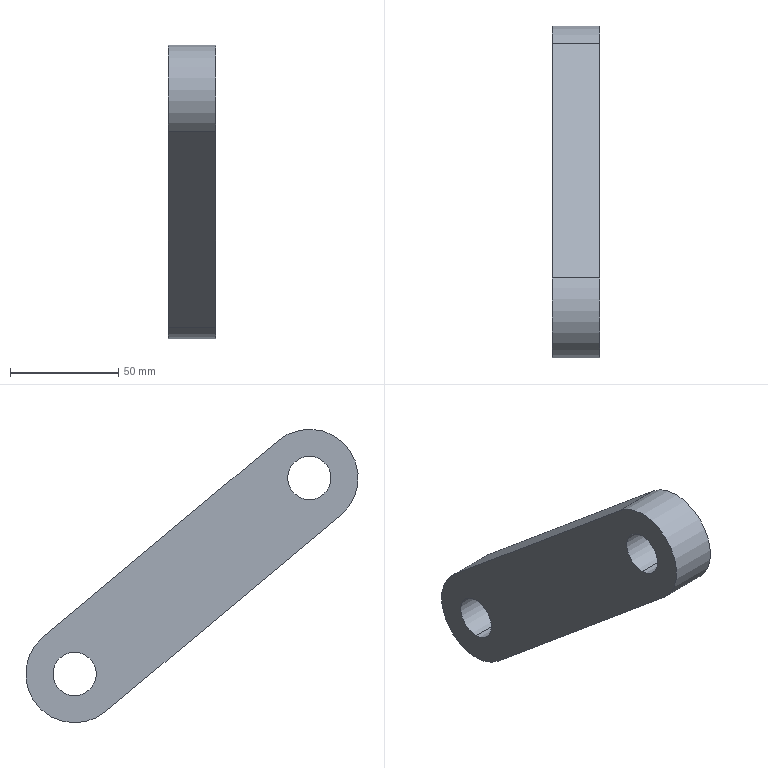Part | SolidWorks | features BaseBody 1, ICE 1, MoveFace 1 | 1 solid | 11 faces | box 22 x 153.344 x 135.399 mm | volume 160860 mm3 | cylinder 7 | plane 4 | commonest cylinder face diameters 20 x4 45 x3
STEP:
#1=CARTESIAN_POINT('',(60.124,30.841,917.301));
#2=VERTEX_POINT('',#1);
#3=CARTESIAN_POINT('',(60.124,30.841,937.301));
#4=VERTEX_POINT('',#3);
#5=CARTESIAN_POINT('',(60.124,30.841,927.301));
#6=DIRECTION('',(-1.,0.,0.));
#7=DIRECTION('',(0.,0.,1.));
#8=AXIS2_PLACEMENT_3D('',#5,#6,#7);
#9=CIRCLE('',#8,10.);
#10=EDGE_CURVE('',#2,#4,#9,.T.);
#11=ORIENTED_EDGE('',*,*,#10,.F.);
#12=CARTESIAN_POINT('',(38.124,30.841,917.301));
#13=VERTEX_POINT('',#12);
#14=CARTESIAN_POINT('',(60.124,30.841,917.301));
#15=DIRECTION('',(-1.,0.,0.));
#16=VECTOR('',#15,1000.);
#17=LINE('',#14,#16);
#18=EDGE_CURVE('',#2,#13,#17,.T.);
#19=ORIENTED_EDGE('',*,*,#18,.T.);
#20=CARTESIAN_POINT('',(38.124,30.841,937.301));
#21=VERTEX_POINT('',#20);
#22=CARTESIAN_POINT('',(38.124,30.841,927.301));
#23=DIRECTION('',(-1.,0.,0.));
#24=DIRECTION('',(0.,0.,1.));
#25=AXIS2_PLACEMENT_3D('',#22,#23,#24);
#26=CIRCLE('',#25,10.);
#27=EDGE_CURVE('',#13,#21,#26,.T.);
#28=ORIENTED_EDGE('',*,*,#27,.T.);
#29=CARTESIAN_POINT('',(60.124,30.841,937.301));
#30=DIRECTION('',(-1.,0.,0.));
#31=VECTOR('',#30,1000.);
#32=LINE('',#29,#31);
#33=EDGE_CURVE('',#4,#21,#32,.T.);
#34=ORIENTED_EDGE('',*,*,#33,.F.);
#35=EDGE_LOOP('',(#11,#19,#28,#34));
#36=FACE_OUTER_BOUND('',#35,.T.);
#37=CARTESIAN_POINT('',(60.124,30.841,927.301));
#38=DIRECTION('',(-1.,0.,0.));
#39=DIRECTION('',(0.,0.,1.));
#40=AXIS2_PLACEMENT_3D('',#37,#38,#39);
#41=CYLINDRICAL_SURFACE('',#40,10.);
#42=ADVANCED_FACE('',(#36),#41,.F.);
#43=CARTESIAN_POINT('',(60.124,-77.503,1007.7));
#44=VERTEX_POINT('',#43);
#45=CARTESIAN_POINT('',(60.124,-77.503,1027.7));
#46=VERTEX_POINT('',#45);
#47=CARTESIAN_POINT('',(60.124,-77.503,1017.7));
#48=DIRECTION('',(-1.,0.,0.));
#49=DIRECTION('',(0.,0.,1.));
#50=AXIS2_PLACEMENT_3D('',#47,#48,#49);
#51=CIRCLE('',#50,10.);
#52=EDGE_CURVE('',#44,#46,#51,.T.);
#53=ORIENTED_EDGE('',*,*,#52,.F.);
#54=CARTESIAN_POINT('',(38.124,-77.503,1007.7));
#55=VERTEX_POINT('',#54);
#56=CARTESIAN_POINT('',(60.124,-77.503,1007.7));
#57=DIRECTION('',(-1.,0.,0.));
#58=VECTOR('',#57,1000.);
#59=LINE('',#56,#58);
#60=EDGE_CURVE('',#44,#55,#59,.T.);
#61=ORIENTED_EDGE('',*,*,#60,.T.);
#62=CARTESIAN_POINT('',(38.124,-77.503,1027.7));
#63=VERTEX_POINT('',#62);
#64=CARTESIAN_POINT('',(38.124,-77.503,1017.7));
#65=DIRECTION('',(-1.,0.,0.));
#66=DIRECTION('',(0.,0.,1.));
#67=AXIS2_PLACEMENT_3D('',#64,#65,#66);
#68=CIRCLE('',#67,10.);
#69=EDGE_CURVE('',#55,#63,#68,.T.);
#70=ORIENTED_EDGE('',*,*,#69,.T.);
#71=CARTESIAN_POINT('',(60.124,-77.503,1027.7));
#72=DIRECTION('',(-1.,0.,0.));
#73=VECTOR('',#72,1000.);
#74=LINE('',#71,#73);
#75=EDGE_CURVE('',#46,#63,#74,.T.);
#76=ORIENTED_EDGE('',*,*,#75,.F.);
#77=EDGE_LOOP('',(#53,#61,#70,#76));
#78=FACE_OUTER_BOUND('',#77,.T.);
#79=CARTESIAN_POINT('',(60.124,-77.503,1017.7));
#80=DIRECTION('',(-1.,0.,0.));
#81=DIRECTION('',(0.,0.,1.));
#82=AXIS2_PLACEMENT_3D('',#79,#80,#81);
#83=CYLINDRICAL_SURFACE('',#82,10.);
#84=ADVANCED_FACE('',(#78),#83,.F.);
#85=CARTESIAN_POINT('',(38.124,16.426,910.025));
#86=VERTEX_POINT('',#85);
#87=CARTESIAN_POINT('',(38.124,30.841,904.801));
#88=VERTEX_POINT('',#87);
#89=CARTESIAN_POINT('',(38.124,30.841,927.301));
#90=DIRECTION('',(1.,0.,0.));
#91=DIRECTION('',(0.,0.,-1.));
#92=AXIS2_PLACEMENT_3D('',#89,#90,#91);
#93=CIRCLE('',#92,22.5);
#94=EDGE_CURVE('',#86,#88,#93,.T.);
#95=ORIENTED_EDGE('',*,*,#94,.T.);
#96=CARTESIAN_POINT('',(60.124,30.841,904.801));
#97=VERTEX_POINT('',#96);
#98=CARTESIAN_POINT('',(48.124,30.841,904.801));
#99=DIRECTION('',(1.,0.,0.));
#100=VECTOR('',#99,1000.);
#101=LINE('',#98,#100);
#102=EDGE_CURVE('',#88,#97,#101,.T.);
#103=ORIENTED_EDGE('',*,*,#102,.T.);
#104=CARTESIAN_POINT('',(60.124,16.426,910.025));
#105=VERTEX_POINT('',#104);
#106=CARTESIAN_POINT('',(60.124,30.841,927.301));
#107=DIRECTION('',(-1.,0.,0.));
#108=DIRECTION('',(0.,0.,-1.));
#109=AXIS2_PLACEMENT_3D('',#106,#107,#108);
#110=CIRCLE('',#109,22.5);
#111=EDGE_CURVE('',#97,#105,#110,.T.);
#112=ORIENTED_EDGE('',*,*,#111,.T.);
#113=CARTESIAN_POINT('',(48.124,16.426,910.025));
#114=DIRECTION('',(-1.,0.,0.));
#115=VECTOR('',#114,1000.);
#116=LINE('',#113,#115);
#117=EDGE_CURVE('',#105,#86,#116,.T.);
#118=ORIENTED_EDGE('',*,*,#117,.T.);
#119=EDGE_LOOP('',(#95,#103,#112,#118));
#120=FACE_OUTER_BOUND('',#119,.T.);
#121=CARTESIAN_POINT('',(48.124,30.841,927.301));
#122=DIRECTION('',(1.,0.,0.));
#123=DIRECTION('',(0.,0.,-1.));
#124=AXIS2_PLACEMENT_3D('',#121,#122,#123);
#125=CYLINDRICAL_SURFACE('',#124,22.5);
#126=ADVANCED_FACE('',(#120),#125,.T.);
#127=CARTESIAN_POINT('',(38.124,30.841,927.301));
#128=DIRECTION('',(-1.,0.,0.));
#129=DIRECTION('',(0.,0.,1.));
#130=AXIS2_PLACEMENT_3D('',#127,#128,#129);
#131=CIRCLE('',#130,10.);
#132=EDGE_CURVE('',#21,#13,#131,.T.);
#133=ORIENTED_EDGE('',*,*,#132,.F.);
#134=ORIENTED_EDGE('',*,*,#27,.F.);
#135=EDGE_LOOP('',(#133,#134));
#136=FACE_BOUND('',#135,.T.);
#137=CARTESIAN_POINT('',(38.124,-77.503,1017.7));
#138=DIRECTION('',(-1.,0.,0.));
#139=DIRECTION('',(0.,0.,1.));
#140=AXIS2_PLACEMENT_3D('',#137,#138,#139);
#141=CIRCLE('',#140,10.);
#142=EDGE_CURVE('',#63,#55,#141,.T.);
#143=ORIENTED_EDGE('',*,*,#142,.F.);
#144=ORIENTED_EDGE('',*,*,#69,.F.);
#145=EDGE_LOOP('',(#143,#144));
#146=FACE_BOUND('',#145,.T.);
#147=ORIENTED_EDGE('',*,*,#94,.F.);
#148=CARTESIAN_POINT('',(38.124,-91.918,1000.424));
#149=VERTEX_POINT('',#148);
#150=CARTESIAN_POINT('',(38.124,-91.918,1000.424));
#151=DIRECTION('',(0.,0.7678,-0.6407));
#152=VECTOR('',#151,1000.);
#153=LINE('',#150,#152);
#154=EDGE_CURVE('',#149,#86,#153,.T.);
#155=ORIENTED_EDGE('',*,*,#154,.F.);
#156=CARTESIAN_POINT('',(38.124,-63.089,1034.976));
#157=VERTEX_POINT('',#156);
#158=CARTESIAN_POINT('',(38.124,-77.503,1017.7));
#159=DIRECTION('',(1.,0.,0.));
#160=DIRECTION('',(0.,0.,-1.));
#161=AXIS2_PLACEMENT_3D('',#158,#159,#160);
#162=CIRCLE('',#161,22.5);
#163=EDGE_CURVE('',#157,#149,#162,.T.);
#164=ORIENTED_EDGE('',*,*,#163,.F.);
#165=CARTESIAN_POINT('',(38.124,45.256,944.577));
#166=VERTEX_POINT('',#165);
#167=CARTESIAN_POINT('',(38.124,45.256,944.577));
#168=DIRECTION('',(0.,-0.7678,0.6407));
#169=VECTOR('',#168,1000.);
#170=LINE('',#167,#169);
#171=EDGE_CURVE('',#166,#157,#170,.T.);
#172=ORIENTED_EDGE('',*,*,#171,.F.);
#173=CARTESIAN_POINT('',(38.124,30.841,927.301));
#174=DIRECTION('',(1.,0.,0.));
#175=DIRECTION('',(0.,0.,-1.));
#176=AXIS2_PLACEMENT_3D('',#173,#174,#175);
#177=CIRCLE('',#176,22.5);
#178=EDGE_CURVE('',#88,#166,#177,.T.);
#179=ORIENTED_EDGE('',*,*,#178,.F.);
#180=EDGE_LOOP('',(#147,#155,#164,#172,#179));
#181=FACE_OUTER_BOUND('',#180,.T.);
#182=CARTESIAN_POINT('',(38.124,30.841,927.301));
#183=DIRECTION('',(1.,0.,0.));
#184=DIRECTION('',(0.,0.,-1.));
#185=AXIS2_PLACEMENT_3D('',#182,#183,#184);
#186=PLANE('',#185);
#187=ADVANCED_FACE('',(#136,#146,#181),#186,.F.);
#188=ORIENTED_EDGE('',*,*,#102,.F.);
#189=ORIENTED_EDGE('',*,*,#178,.T.);
#190=CARTESIAN_POINT('',(60.124,45.256,944.577));
#191=VERTEX_POINT('',#190);
#192=CARTESIAN_POINT('',(48.124,45.256,944.577));
#193=DIRECTION('',(1.,0.,0.));
#194=VECTOR('',#193,1000.);
#195=LINE('',#192,#194);
#196=EDGE_CURVE('',#166,#191,#195,.T.);
#197=ORIENTED_EDGE('',*,*,#196,.T.);
#198=CARTESIAN_POINT('',(60.124,30.841,927.301));
#199=DIRECTION('',(-1.,0.,0.));
#200=DIRECTION('',(0.,0.,-1.));
#201=AXIS2_PLACEMENT_3D('',#198,#199,#200);
#202=CIRCLE('',#201,22.5);
#203=EDGE_CURVE('',#191,#97,#202,.T.);
#204=ORIENTED_EDGE('',*,*,#203,.T.);
#205=EDGE_LOOP('',(#188,#189,#197,#204));
#206=FACE_OUTER_BOUND('',#205,.T.);
#207=CARTESIAN_POINT('',(48.124,30.841,927.301));
#208=DIRECTION('',(1.,0.,0.));
#209=DIRECTION('',(0.,0.,-1.));
#210=AXIS2_PLACEMENT_3D('',#207,#208,#209);
#211=CYLINDRICAL_SURFACE('',#210,22.5);
#212=ADVANCED_FACE('',(#206),#211,.T.);
#213=CARTESIAN_POINT('',(60.124,-91.918,1000.424));
#214=VERTEX_POINT('',#213);
#215=CARTESIAN_POINT('',(48.124,-91.918,1000.424));
#216=DIRECTION('',(1.,0.,0.));
#217=VECTOR('',#216,1000.);
#218=LINE('',#215,#217);
#219=EDGE_CURVE('',#149,#214,#218,.T.);
#220=ORIENTED_EDGE('',*,*,#219,.F.);
#221=ORIENTED_EDGE('',*,*,#154,.T.);
#222=ORIENTED_EDGE('',*,*,#117,.F.);
#223=CARTESIAN_POINT('',(60.124,16.426,910.025));
#224=DIRECTION('',(0.,0.7678,-0.6407));
#225=VECTOR('',#224,1000.);
#226=LINE('',#223,#225);
#227=EDGE_CURVE('',#214,#105,#226,.T.);
#228=ORIENTED_EDGE('',*,*,#227,.F.);
#229=EDGE_LOOP('',(#220,#221,#222,#228));
#230=FACE_OUTER_BOUND('',#229,.T.);
#231=CARTESIAN_POINT('',(48.124,16.426,910.025));
#232=DIRECTION('',(0.,0.6407,0.7678));
#233=DIRECTION('',(0.,-0.7678,0.6407));
#234=AXIS2_PLACEMENT_3D('',#231,#232,#233);
#235=PLANE('',#234);
#236=ADVANCED_FACE('',(#230),#235,.F.);
#237=ORIENTED_EDGE('',*,*,#163,.T.);
#238=ORIENTED_EDGE('',*,*,#219,.T.);
#239=CARTESIAN_POINT('',(60.124,-63.089,1034.976));
#240=VERTEX_POINT('',#239);
#241=CARTESIAN_POINT('',(60.124,-77.503,1017.7));
#242=DIRECTION('',(-1.,0.,0.));
#243=DIRECTION('',(0.,0.,-1.));
#244=AXIS2_PLACEMENT_3D('',#241,#242,#243);
#245=CIRCLE('',#244,22.5);
#246=EDGE_CURVE('',#214,#240,#245,.T.);
#247=ORIENTED_EDGE('',*,*,#246,.T.);
#248=CARTESIAN_POINT('',(48.124,-63.089,1034.976));
#249=DIRECTION('',(-1.,0.,0.));
#250=VECTOR('',#249,1000.);
#251=LINE('',#248,#250);
#252=EDGE_CURVE('',#240,#157,#251,.T.);
#253=ORIENTED_EDGE('',*,*,#252,.T.);
#254=EDGE_LOOP('',(#237,#238,#247,#253));
#255=FACE_OUTER_BOUND('',#254,.T.);
#256=CARTESIAN_POINT('',(48.124,-77.503,1017.7));
#257=DIRECTION('',(1.,0.,0.));
#258=DIRECTION('',(0.,0.,-1.));
#259=AXIS2_PLACEMENT_3D('',#256,#257,#258);
#260=CYLINDRICAL_SURFACE('',#259,22.5);
#261=ADVANCED_FACE('',(#255),#260,.T.);
#262=ORIENTED_EDGE('',*,*,#196,.F.);
#263=ORIENTED_EDGE('',*,*,#171,.T.);
#264=ORIENTED_EDGE('',*,*,#252,.F.);
#265=CARTESIAN_POINT('',(60.124,45.256,944.577));
#266=DIRECTION('',(0.,-0.7678,0.6407));
#267=VECTOR('',#266,1000.);
#268=LINE('',#265,#267);
#269=EDGE_CURVE('',#191,#240,#268,.T.);
#270=ORIENTED_EDGE('',*,*,#269,.F.);
#271=EDGE_LOOP('',(#262,#263,#264,#270));
#272=FACE_OUTER_BOUND('',#271,.T.);
#273=CARTESIAN_POINT('',(48.124,45.256,944.577));
#274=DIRECTION('',(0.,-0.6407,-0.7678));
#275=DIRECTION('',(0.,0.7678,-0.6407));
#276=AXIS2_PLACEMENT_3D('',#273,#274,#275);
#277=PLANE('',#276);
#278=ADVANCED_FACE('',(#272),#277,.F.);
#279=CARTESIAN_POINT('',(60.124,30.841,927.301));
#280=DIRECTION('',(-1.,0.,0.));
#281=DIRECTION('',(0.,0.,1.));
#282=AXIS2_PLACEMENT_3D('',#279,#280,#281);
#283=CIRCLE('',#282,10.);
#284=EDGE_CURVE('',#4,#2,#283,.T.);
#285=ORIENTED_EDGE('',*,*,#284,.T.);
#286=ORIENTED_EDGE('',*,*,#10,.T.);
#287=EDGE_LOOP('',(#285,#286));
#288=FACE_BOUND('',#287,.T.);
#289=CARTESIAN_POINT('',(60.124,-77.503,1017.7));
#290=DIRECTION('',(-1.,0.,0.));
#291=DIRECTION('',(0.,0.,1.));
#292=AXIS2_PLACEMENT_3D('',#289,#290,#291);
#293=CIRCLE('',#292,10.);
#294=EDGE_CURVE('',#46,#44,#293,.T.);
#295=ORIENTED_EDGE('',*,*,#294,.T.);
#296=ORIENTED_EDGE('',*,*,#52,.T.);
#297=EDGE_LOOP('',(#295,#296));
#298=FACE_BOUND('',#297,.T.);
#299=ORIENTED_EDGE('',*,*,#227,.T.);
#300=ORIENTED_EDGE('',*,*,#111,.F.);
#301=ORIENTED_EDGE('',*,*,#203,.F.);
#302=ORIENTED_EDGE('',*,*,#269,.T.);
#303=ORIENTED_EDGE('',*,*,#246,.F.);
#304=EDGE_LOOP('',(#299,#300,#301,#302,#303));
#305=FACE_OUTER_BOUND('',#304,.T.);
#306=CARTESIAN_POINT('',(60.124,30.841,927.301));
#307=DIRECTION('',(1.,0.,0.));
#308=DIRECTION('',(0.,0.,-1.));
#309=AXIS2_PLACEMENT_3D('',#306,#307,#308);
#310=PLANE('',#309);
#311=ADVANCED_FACE('',(#288,#298,#305),#310,.T.);
#312=ORIENTED_EDGE('',*,*,#60,.F.);
#313=ORIENTED_EDGE('',*,*,#294,.F.);
#314=ORIENTED_EDGE('',*,*,#75,.T.);
#315=ORIENTED_EDGE('',*,*,#142,.T.);
#316=EDGE_LOOP('',(#312,#313,#314,#315));
#317=FACE_OUTER_BOUND('',#316,.T.);
#318=CARTESIAN_POINT('',(60.124,-77.503,1017.7));
#319=DIRECTION('',(-1.,0.,0.));
#320=DIRECTION('',(0.,0.,1.));
#321=AXIS2_PLACEMENT_3D('',#318,#319,#320);
#322=CYLINDRICAL_SURFACE('',#321,10.);
#323=ADVANCED_FACE('',(#317),#322,.F.);
#324=ORIENTED_EDGE('',*,*,#18,.F.);
#325=ORIENTED_EDGE('',*,*,#284,.F.);
#326=ORIENTED_EDGE('',*,*,#33,.T.);
#327=ORIENTED_EDGE('',*,*,#132,.T.);
#328=EDGE_LOOP('',(#324,#325,#326,#327));
#329=FACE_OUTER_BOUND('',#328,.T.);
#330=CARTESIAN_POINT('',(60.124,30.841,927.301));
#331=DIRECTION('',(-1.,0.,0.));
#332=DIRECTION('',(0.,0.,1.));
#333=AXIS2_PLACEMENT_3D('',#330,#331,#332);
#334=CYLINDRICAL_SURFACE('',#333,10.);
#335=ADVANCED_FACE('',(#329),#334,.F.);
#336=CLOSED_SHELL('',(#42,#84,#126,#187,#212,#236,#261,#278,#311,#323,#335));
#337=MANIFOLD_SOLID_BREP('',#336);
#338=CARTESIAN_POINT('',(0.,0.,0.));
#339=DIRECTION('',(0.,0.,1.));
#340=DIRECTION('',(1.,0.,0.));
#341=AXIS2_PLACEMENT_3D('',#338,#339,#340);
#342=(LENGTH_UNIT()NAMED_UNIT(*)SI_UNIT(.MILLI.,.METRE.));
#343=UNCERTAINTY_MEASURE_WITH_UNIT(LENGTH_MEASURE(0.00001),#342,'','');
#344=(NAMED_UNIT(*)PLANE_ANGLE_UNIT()SI_UNIT($,.RADIAN.));
#345=(NAMED_UNIT(*)SI_UNIT($,.STERADIAN.)SOLID_ANGLE_UNIT());
#346=(GEOMETRIC_REPRESENTATION_CONTEXT(3)GLOBAL_UNCERTAINTY_ASSIGNED_CONTEXT((#343))GLOBAL_UNIT_ASSIGNED_CONTEXT((#342,#344,#345))REPRESENTATION_CONTEXT('',''));
#347=ADVANCED_BREP_SHAPE_REPRESENTATION('',(#337,#341),#346);